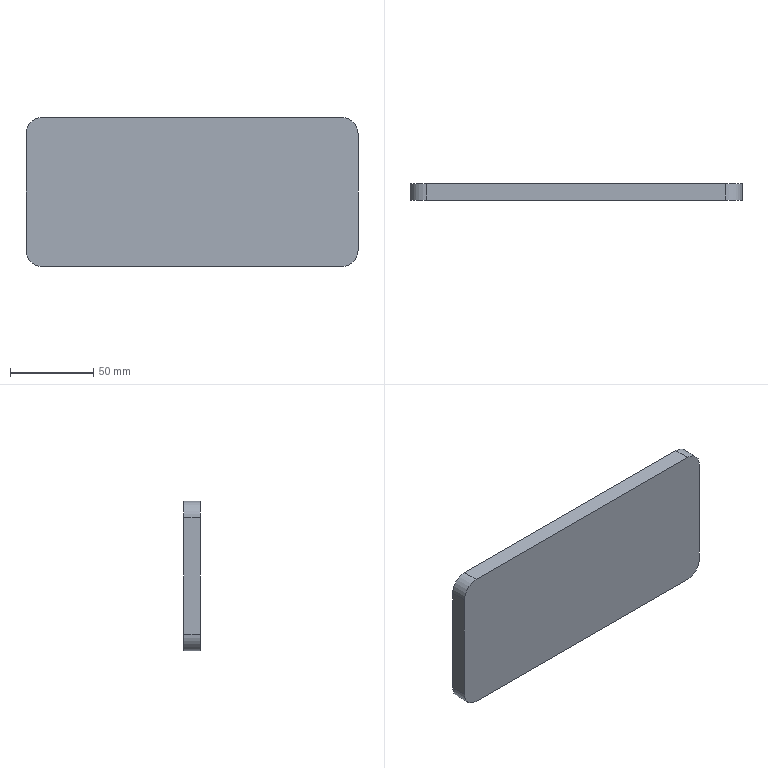Part | SolidWorks | features Extrusion 1, Fillet 1 | 1 solid | 10 faces | box 200 x 10 x 90 mm | volume 179142 mm3 | plane 6 | cylinder 4 | commonest cylinder face diameters 20 x4
STEP:
#1=CARTESIAN_POINT('',(0.,10.,-80.));
#2=VERTEX_POINT('',#1);
#3=CARTESIAN_POINT('',(0.,10.,-10.));
#4=VERTEX_POINT('',#3);
#5=CARTESIAN_POINT('',(0.,10.,0.));
#6=DIRECTION('',(0.,0.,1.));
#7=VECTOR('',#6,1000.);
#8=LINE('',#5,#7);
#9=EDGE_CURVE('',#2,#4,#8,.T.);
#10=ORIENTED_EDGE('',*,*,#9,.F.);
#11=CARTESIAN_POINT('',(0.,0.,-80.));
#12=VERTEX_POINT('',#11);
#13=CARTESIAN_POINT('',(0.,10.,-80.));
#14=DIRECTION('',(0.,-1.,0.));
#15=VECTOR('',#14,1000.);
#16=LINE('',#13,#15);
#17=EDGE_CURVE('',#2,#12,#16,.T.);
#18=ORIENTED_EDGE('',*,*,#17,.T.);
#19=CARTESIAN_POINT('',(0.,0.,-10.));
#20=VERTEX_POINT('',#19);
#21=CARTESIAN_POINT('',(0.,0.,0.));
#22=DIRECTION('',(0.,0.,1.));
#23=VECTOR('',#22,1000.);
#24=LINE('',#21,#23);
#25=EDGE_CURVE('',#12,#20,#24,.T.);
#26=ORIENTED_EDGE('',*,*,#25,.T.);
#27=CARTESIAN_POINT('',(0.,10.,-10.));
#28=DIRECTION('',(0.,1.,0.));
#29=VECTOR('',#28,1000.);
#30=LINE('',#27,#29);
#31=EDGE_CURVE('',#20,#4,#30,.T.);
#32=ORIENTED_EDGE('',*,*,#31,.T.);
#33=EDGE_LOOP('',(#10,#18,#26,#32));
#34=FACE_OUTER_BOUND('',#33,.T.);
#35=CARTESIAN_POINT('',(0.,10.,0.));
#36=DIRECTION('',(1.,0.,0.));
#37=DIRECTION('',(0.,0.,-1.));
#38=AXIS2_PLACEMENT_3D('',#35,#36,#37);
#39=PLANE('',#38);
#40=ADVANCED_FACE('',(#34),#39,.F.);
#41=CARTESIAN_POINT('',(10.,10.,0.));
#42=VERTEX_POINT('',#41);
#43=CARTESIAN_POINT('',(190.,10.,0.));
#44=VERTEX_POINT('',#43);
#45=CARTESIAN_POINT('',(0.,10.,0.));
#46=DIRECTION('',(1.,0.,0.));
#47=VECTOR('',#46,1000.);
#48=LINE('',#45,#47);
#49=EDGE_CURVE('',#42,#44,#48,.T.);
#50=ORIENTED_EDGE('',*,*,#49,.F.);
#51=CARTESIAN_POINT('',(10.,0.,0.));
#52=VERTEX_POINT('',#51);
#53=CARTESIAN_POINT('',(10.,10.,0.));
#54=DIRECTION('',(0.,-1.,0.));
#55=VECTOR('',#54,1000.);
#56=LINE('',#53,#55);
#57=EDGE_CURVE('',#42,#52,#56,.T.);
#58=ORIENTED_EDGE('',*,*,#57,.T.);
#59=CARTESIAN_POINT('',(190.,0.,0.));
#60=VERTEX_POINT('',#59);
#61=CARTESIAN_POINT('',(0.,0.,0.));
#62=DIRECTION('',(1.,0.,0.));
#63=VECTOR('',#62,1000.);
#64=LINE('',#61,#63);
#65=EDGE_CURVE('',#52,#60,#64,.T.);
#66=ORIENTED_EDGE('',*,*,#65,.T.);
#67=CARTESIAN_POINT('',(190.,10.,0.));
#68=DIRECTION('',(0.,1.,0.));
#69=VECTOR('',#68,1000.);
#70=LINE('',#67,#69);
#71=EDGE_CURVE('',#60,#44,#70,.T.);
#72=ORIENTED_EDGE('',*,*,#71,.T.);
#73=EDGE_LOOP('',(#50,#58,#66,#72));
#74=FACE_OUTER_BOUND('',#73,.T.);
#75=CARTESIAN_POINT('',(0.,10.,0.));
#76=DIRECTION('',(0.,0.,-1.));
#77=DIRECTION('',(-1.,0.,0.));
#78=AXIS2_PLACEMENT_3D('',#75,#76,#77);
#79=PLANE('',#78);
#80=ADVANCED_FACE('',(#74),#79,.F.);
#81=CARTESIAN_POINT('',(200.,0.,-10.));
#82=VERTEX_POINT('',#81);
#83=CARTESIAN_POINT('',(200.,0.,-80.));
#84=VERTEX_POINT('',#83);
#85=CARTESIAN_POINT('',(200.,0.,0.));
#86=DIRECTION('',(0.,0.,-1.));
#87=VECTOR('',#86,1000.);
#88=LINE('',#85,#87);
#89=EDGE_CURVE('',#82,#84,#88,.T.);
#90=ORIENTED_EDGE('',*,*,#89,.T.);
#91=CARTESIAN_POINT('',(200.,10.,-80.));
#92=VERTEX_POINT('',#91);
#93=CARTESIAN_POINT('',(200.,10.,-80.));
#94=DIRECTION('',(0.,1.,0.));
#95=VECTOR('',#94,1000.);
#96=LINE('',#93,#95);
#97=EDGE_CURVE('',#84,#92,#96,.T.);
#98=ORIENTED_EDGE('',*,*,#97,.T.);
#99=CARTESIAN_POINT('',(200.,10.,-10.));
#100=VERTEX_POINT('',#99);
#101=CARTESIAN_POINT('',(200.,10.,0.));
#102=DIRECTION('',(0.,0.,-1.));
#103=VECTOR('',#102,1000.);
#104=LINE('',#101,#103);
#105=EDGE_CURVE('',#100,#92,#104,.T.);
#106=ORIENTED_EDGE('',*,*,#105,.F.);
#107=CARTESIAN_POINT('',(200.,10.,-10.));
#108=DIRECTION('',(0.,-1.,0.));
#109=VECTOR('',#108,1000.);
#110=LINE('',#107,#109);
#111=EDGE_CURVE('',#100,#82,#110,.T.);
#112=ORIENTED_EDGE('',*,*,#111,.T.);
#113=EDGE_LOOP('',(#90,#98,#106,#112));
#114=FACE_OUTER_BOUND('',#113,.T.);
#115=CARTESIAN_POINT('',(200.,10.,0.));
#116=DIRECTION('',(-1.,0.,0.));
#117=DIRECTION('',(0.,0.,1.));
#118=AXIS2_PLACEMENT_3D('',#115,#116,#117);
#119=PLANE('',#118);
#120=ADVANCED_FACE('',(#114),#119,.F.);
#121=CARTESIAN_POINT('',(190.,0.,-90.));
#122=VERTEX_POINT('',#121);
#123=CARTESIAN_POINT('',(10.,0.,-90.));
#124=VERTEX_POINT('',#123);
#125=CARTESIAN_POINT('',(0.,0.,-90.));
#126=DIRECTION('',(-1.,0.,0.));
#127=VECTOR('',#126,1000.);
#128=LINE('',#125,#127);
#129=EDGE_CURVE('',#122,#124,#128,.T.);
#130=ORIENTED_EDGE('',*,*,#129,.T.);
#131=CARTESIAN_POINT('',(10.,10.,-90.));
#132=VERTEX_POINT('',#131);
#133=CARTESIAN_POINT('',(10.,10.,-90.));
#134=DIRECTION('',(0.,1.,0.));
#135=VECTOR('',#134,1000.);
#136=LINE('',#133,#135);
#137=EDGE_CURVE('',#124,#132,#136,.T.);
#138=ORIENTED_EDGE('',*,*,#137,.T.);
#139=CARTESIAN_POINT('',(190.,10.,-90.));
#140=VERTEX_POINT('',#139);
#141=CARTESIAN_POINT('',(0.,10.,-90.));
#142=DIRECTION('',(-1.,0.,0.));
#143=VECTOR('',#142,1000.);
#144=LINE('',#141,#143);
#145=EDGE_CURVE('',#140,#132,#144,.T.);
#146=ORIENTED_EDGE('',*,*,#145,.F.);
#147=CARTESIAN_POINT('',(190.,10.,-90.));
#148=DIRECTION('',(0.,-1.,0.));
#149=VECTOR('',#148,1000.);
#150=LINE('',#147,#149);
#151=EDGE_CURVE('',#140,#122,#150,.T.);
#152=ORIENTED_EDGE('',*,*,#151,.T.);
#153=EDGE_LOOP('',(#130,#138,#146,#152));
#154=FACE_OUTER_BOUND('',#153,.T.);
#155=CARTESIAN_POINT('',(0.,10.,-90.));
#156=DIRECTION('',(0.,0.,1.));
#157=DIRECTION('',(1.,0.,0.));
#158=AXIS2_PLACEMENT_3D('',#155,#156,#157);
#159=PLANE('',#158);
#160=ADVANCED_FACE('',(#154),#159,.F.);
#161=ORIENTED_EDGE('',*,*,#145,.T.);
#162=CARTESIAN_POINT('',(10.,10.,-80.));
#163=DIRECTION('',(0.,1.,0.));
#164=DIRECTION('',(0.,0.,-1.));
#165=AXIS2_PLACEMENT_3D('',#162,#163,#164);
#166=CIRCLE('',#165,10.);
#167=EDGE_CURVE('',#132,#2,#166,.T.);
#168=ORIENTED_EDGE('',*,*,#167,.T.);
#169=ORIENTED_EDGE('',*,*,#9,.T.);
#170=CARTESIAN_POINT('',(10.,10.,-10.));
#171=DIRECTION('',(0.,1.,0.));
#172=DIRECTION('',(0.,0.,-1.));
#173=AXIS2_PLACEMENT_3D('',#170,#171,#172);
#174=CIRCLE('',#173,10.);
#175=EDGE_CURVE('',#4,#42,#174,.T.);
#176=ORIENTED_EDGE('',*,*,#175,.T.);
#177=ORIENTED_EDGE('',*,*,#49,.T.);
#178=CARTESIAN_POINT('',(190.,10.,-10.));
#179=DIRECTION('',(0.,1.,0.));
#180=DIRECTION('',(0.,0.,-1.));
#181=AXIS2_PLACEMENT_3D('',#178,#179,#180);
#182=CIRCLE('',#181,10.);
#183=EDGE_CURVE('',#44,#100,#182,.T.);
#184=ORIENTED_EDGE('',*,*,#183,.T.);
#185=ORIENTED_EDGE('',*,*,#105,.T.);
#186=CARTESIAN_POINT('',(190.,10.,-80.));
#187=DIRECTION('',(0.,1.,0.));
#188=DIRECTION('',(0.,0.,-1.));
#189=AXIS2_PLACEMENT_3D('',#186,#187,#188);
#190=CIRCLE('',#189,10.);
#191=EDGE_CURVE('',#92,#140,#190,.T.);
#192=ORIENTED_EDGE('',*,*,#191,.T.);
#193=EDGE_LOOP('',(#161,#168,#169,#176,#177,#184,#185,#192));
#194=FACE_OUTER_BOUND('',#193,.T.);
#195=CARTESIAN_POINT('',(0.,10.,0.));
#196=DIRECTION('',(0.,-1.,0.));
#197=DIRECTION('',(0.,0.,-1.));
#198=AXIS2_PLACEMENT_3D('',#195,#196,#197);
#199=PLANE('',#198);
#200=ADVANCED_FACE('',(#194),#199,.F.);
#201=ORIENTED_EDGE('',*,*,#25,.F.);
#202=CARTESIAN_POINT('',(10.,0.,-80.));
#203=DIRECTION('',(0.,-1.,0.));
#204=DIRECTION('',(0.,0.,-1.));
#205=AXIS2_PLACEMENT_3D('',#202,#203,#204);
#206=CIRCLE('',#205,10.);
#207=EDGE_CURVE('',#12,#124,#206,.T.);
#208=ORIENTED_EDGE('',*,*,#207,.T.);
#209=ORIENTED_EDGE('',*,*,#129,.F.);
#210=CARTESIAN_POINT('',(190.,0.,-80.));
#211=DIRECTION('',(0.,-1.,0.));
#212=DIRECTION('',(0.,0.,-1.));
#213=AXIS2_PLACEMENT_3D('',#210,#211,#212);
#214=CIRCLE('',#213,10.);
#215=EDGE_CURVE('',#122,#84,#214,.T.);
#216=ORIENTED_EDGE('',*,*,#215,.T.);
#217=ORIENTED_EDGE('',*,*,#89,.F.);
#218=CARTESIAN_POINT('',(190.,0.,-10.));
#219=DIRECTION('',(0.,-1.,0.));
#220=DIRECTION('',(0.,0.,-1.));
#221=AXIS2_PLACEMENT_3D('',#218,#219,#220);
#222=CIRCLE('',#221,10.);
#223=EDGE_CURVE('',#82,#60,#222,.T.);
#224=ORIENTED_EDGE('',*,*,#223,.T.);
#225=ORIENTED_EDGE('',*,*,#65,.F.);
#226=CARTESIAN_POINT('',(10.,0.,-10.));
#227=DIRECTION('',(0.,-1.,0.));
#228=DIRECTION('',(0.,0.,-1.));
#229=AXIS2_PLACEMENT_3D('',#226,#227,#228);
#230=CIRCLE('',#229,10.);
#231=EDGE_CURVE('',#52,#20,#230,.T.);
#232=ORIENTED_EDGE('',*,*,#231,.T.);
#233=EDGE_LOOP('',(#201,#208,#209,#216,#217,#224,#225,#232));
#234=FACE_OUTER_BOUND('',#233,.T.);
#235=CARTESIAN_POINT('',(0.,0.,0.));
#236=DIRECTION('',(0.,-1.,0.));
#237=DIRECTION('',(0.,0.,-1.));
#238=AXIS2_PLACEMENT_3D('',#235,#236,#237);
#239=PLANE('',#238);
#240=ADVANCED_FACE('',(#234),#239,.T.);
#241=ORIENTED_EDGE('',*,*,#167,.F.);
#242=ORIENTED_EDGE('',*,*,#137,.F.);
#243=ORIENTED_EDGE('',*,*,#207,.F.);
#244=ORIENTED_EDGE('',*,*,#17,.F.);
#245=EDGE_LOOP('',(#241,#242,#243,#244));
#246=FACE_OUTER_BOUND('',#245,.T.);
#247=CARTESIAN_POINT('',(10.,10.,-80.));
#248=DIRECTION('',(0.,-1.,0.));
#249=DIRECTION('',(0.,0.,-1.));
#250=AXIS2_PLACEMENT_3D('',#247,#248,#249);
#251=CYLINDRICAL_SURFACE('',#250,10.);
#252=ADVANCED_FACE('',(#246),#251,.T.);
#253=ORIENTED_EDGE('',*,*,#175,.F.);
#254=ORIENTED_EDGE('',*,*,#31,.F.);
#255=ORIENTED_EDGE('',*,*,#231,.F.);
#256=ORIENTED_EDGE('',*,*,#57,.F.);
#257=EDGE_LOOP('',(#253,#254,#255,#256));
#258=FACE_OUTER_BOUND('',#257,.T.);
#259=CARTESIAN_POINT('',(10.,10.,-10.));
#260=DIRECTION('',(0.,-1.,0.));
#261=DIRECTION('',(0.,0.,-1.));
#262=AXIS2_PLACEMENT_3D('',#259,#260,#261);
#263=CYLINDRICAL_SURFACE('',#262,10.);
#264=ADVANCED_FACE('',(#258),#263,.T.);
#265=ORIENTED_EDGE('',*,*,#191,.F.);
#266=ORIENTED_EDGE('',*,*,#97,.F.);
#267=ORIENTED_EDGE('',*,*,#215,.F.);
#268=ORIENTED_EDGE('',*,*,#151,.F.);
#269=EDGE_LOOP('',(#265,#266,#267,#268));
#270=FACE_OUTER_BOUND('',#269,.T.);
#271=CARTESIAN_POINT('',(190.,10.,-80.));
#272=DIRECTION('',(0.,-1.,0.));
#273=DIRECTION('',(0.,0.,-1.));
#274=AXIS2_PLACEMENT_3D('',#271,#272,#273);
#275=CYLINDRICAL_SURFACE('',#274,10.);
#276=ADVANCED_FACE('',(#270),#275,.T.);
#277=ORIENTED_EDGE('',*,*,#183,.F.);
#278=ORIENTED_EDGE('',*,*,#71,.F.);
#279=ORIENTED_EDGE('',*,*,#223,.F.);
#280=ORIENTED_EDGE('',*,*,#111,.F.);
#281=EDGE_LOOP('',(#277,#278,#279,#280));
#282=FACE_OUTER_BOUND('',#281,.T.);
#283=CARTESIAN_POINT('',(190.,10.,-10.));
#284=DIRECTION('',(0.,-1.,0.));
#285=DIRECTION('',(0.,0.,-1.));
#286=AXIS2_PLACEMENT_3D('',#283,#284,#285);
#287=CYLINDRICAL_SURFACE('',#286,10.);
#288=ADVANCED_FACE('',(#282),#287,.T.);
#289=CLOSED_SHELL('',(#40,#80,#120,#160,#200,#240,#252,#264,#276,#288));
#290=MANIFOLD_SOLID_BREP('',#289);
#291=CARTESIAN_POINT('',(0.,0.,0.));
#292=DIRECTION('',(0.,0.,1.));
#293=DIRECTION('',(1.,0.,0.));
#294=AXIS2_PLACEMENT_3D('',#291,#292,#293);
#295=(LENGTH_UNIT()NAMED_UNIT(*)SI_UNIT(.MILLI.,.METRE.));
#296=UNCERTAINTY_MEASURE_WITH_UNIT(LENGTH_MEASURE(0.00001),#295,'','');
#297=(NAMED_UNIT(*)PLANE_ANGLE_UNIT()SI_UNIT($,.RADIAN.));
#298=(NAMED_UNIT(*)SI_UNIT($,.STERADIAN.)SOLID_ANGLE_UNIT());
#299=(GEOMETRIC_REPRESENTATION_CONTEXT(3)GLOBAL_UNCERTAINTY_ASSIGNED_CONTEXT((#296))GLOBAL_UNIT_ASSIGNED_CONTEXT((#295,#297,#298))REPRESENTATION_CONTEXT('',''));
#300=ADVANCED_BREP_SHAPE_REPRESENTATION('',(#290,#294),#299);